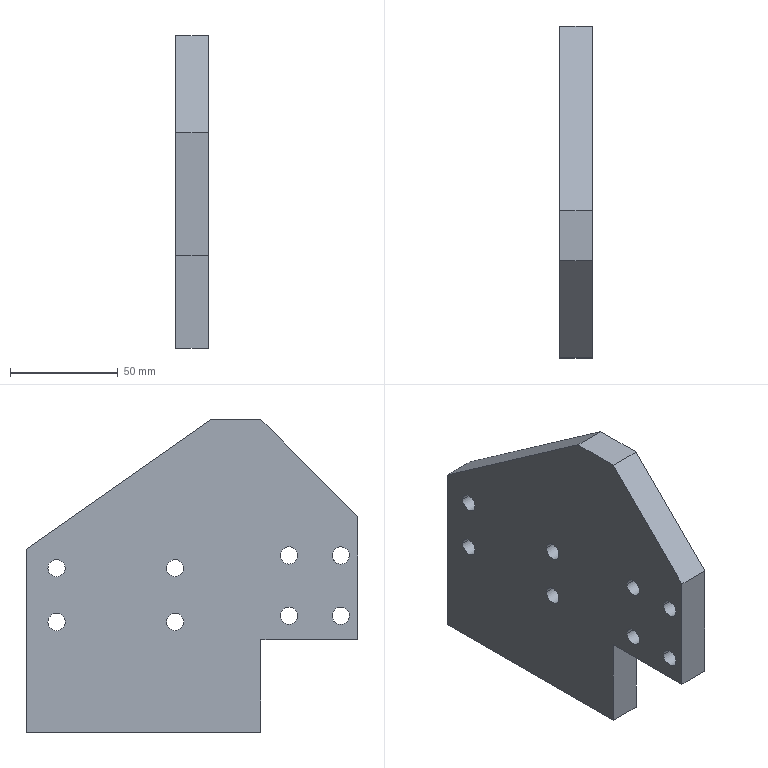Part | STEP file | Positioning_id1402_x_t | 1 solid | 26 faces | box 15 x 154 x 145 mm | volume 246102 mm3 | cylinder 16 | plane 10 | commonest cylinder face diameters 8 x16